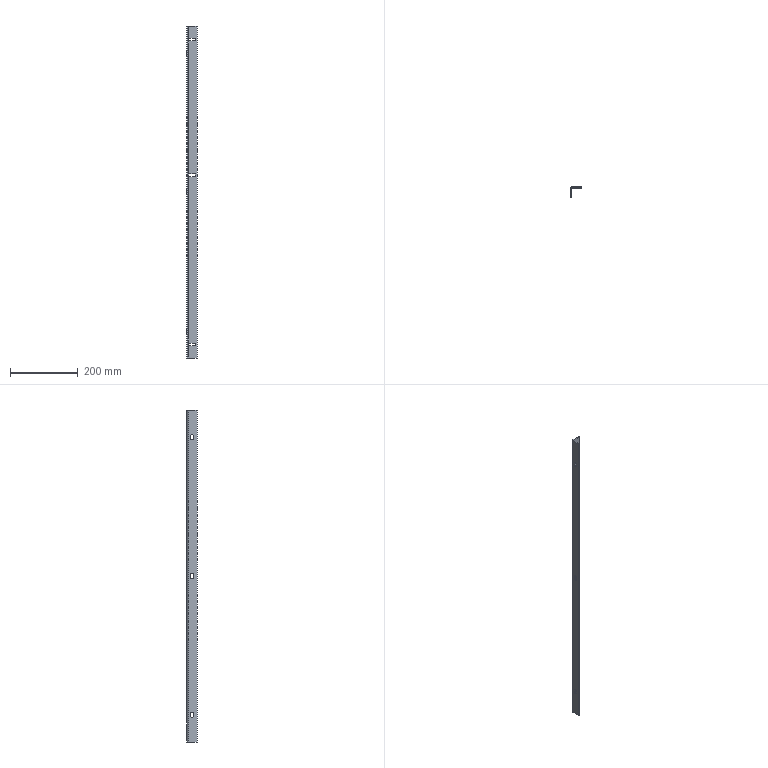Part | NX | features solid 2 | 1 solid | 34 faces | box 30 x 30 x 980 mm | volume 134896 mm3 | plane 26 | cylinder 8 | commonest cylinder face diameters 7 x6 5 x1 10 x1
STEP:
#1=CARTESIAN_POINT('',(-320.,497.5,311.25));
#2=VERTEX_POINT('',#1);
#3=CARTESIAN_POINT('',(-320.,500.,311.25));
#4=VERTEX_POINT('',#3);
#5=CARTESIAN_POINT('',(-320.,-480.918,311.25));
#6=DIRECTION('',(0.,1.,0.));
#7=VECTOR('',#6,1000.);
#8=LINE('',#5,#7);
#9=EDGE_CURVE('',#2,#4,#8,.T.);
#10=ORIENTED_EDGE('',*,*,#9,.T.);
#11=CARTESIAN_POINT('',(-300.,500.,311.25));
#12=VERTEX_POINT('',#11);
#13=CARTESIAN_POINT('',(-320.,500.,311.25));
#14=DIRECTION('',(1.,0.,0.));
#15=VECTOR('',#14,1000.);
#16=LINE('',#13,#15);
#17=EDGE_CURVE('',#4,#12,#16,.T.);
#18=ORIENTED_EDGE('',*,*,#17,.T.);
#19=CARTESIAN_POINT('',(-300.,497.5,311.25));
#20=VERTEX_POINT('',#19);
#21=CARTESIAN_POINT('',(-300.,-480.918,311.25));
#22=DIRECTION('',(0.,1.,0.));
#23=VECTOR('',#22,1000.);
#24=LINE('',#21,#23);
#25=EDGE_CURVE('',#20,#12,#24,.T.);
#26=ORIENTED_EDGE('',*,*,#25,.F.);
#27=CARTESIAN_POINT('',(-295.,497.5,311.25));
#28=DIRECTION('',(1.,0.,0.));
#29=VECTOR('',#28,1000.);
#30=LINE('',#27,#29);
#31=EDGE_CURVE('',#2,#20,#30,.T.);
#32=ORIENTED_EDGE('',*,*,#31,.F.);
#33=EDGE_LOOP('',(#10,#18,#26,#32));
#34=FACE_BOUND('',#33,.T.);
#35=CARTESIAN_POINT('',(-320.,-480.918,311.25));
#36=DIRECTION('',(0.,0.,1.));
#37=DIRECTION('',(1.,0.,0.));
#38=AXIS2_PLACEMENT_3D('',#35,#36,#37);
#39=PLANE('',#38);
#40=ADVANCED_FACE('',(#34),#39,.F.);
#41=CARTESIAN_POINT('',(-320.,497.5,302.75));
#42=VERTEX_POINT('',#41);
#43=CARTESIAN_POINT('',(-320.,500.,302.75));
#44=VERTEX_POINT('',#43);
#45=CARTESIAN_POINT('',(-320.,-480.918,302.75));
#46=DIRECTION('',(0.,1.,0.));
#47=VECTOR('',#46,1000.);
#48=LINE('',#45,#47);
#49=EDGE_CURVE('',#42,#44,#48,.T.);
#50=ORIENTED_EDGE('',*,*,#49,.T.);
#51=CARTESIAN_POINT('',(-320.,500.,311.25));
#52=DIRECTION('',(0.,0.,1.));
#53=VECTOR('',#52,1000.);
#54=LINE('',#51,#53);
#55=EDGE_CURVE('',#44,#4,#54,.T.);
#56=ORIENTED_EDGE('',*,*,#55,.T.);
#57=ORIENTED_EDGE('',*,*,#9,.F.);
#58=CARTESIAN_POINT('',(-320.,497.5,267.));
#59=DIRECTION('',(0.,0.,1.));
#60=VECTOR('',#59,1000.);
#61=LINE('',#58,#60);
#62=EDGE_CURVE('',#42,#2,#61,.T.);
#63=ORIENTED_EDGE('',*,*,#62,.F.);
#64=EDGE_LOOP('',(#50,#56,#57,#63));
#65=FACE_BOUND('',#64,.T.);
#66=CARTESIAN_POINT('',(-320.,-480.918,311.25));
#67=DIRECTION('',(-1.,0.,0.));
#68=DIRECTION('',(0.,1.,0.));
#69=AXIS2_PLACEMENT_3D('',#66,#67,#68);
#70=PLANE('',#69);
#71=ADVANCED_FACE('',(#65),#70,.F.);
#72=CARTESIAN_POINT('',(-300.,497.5,302.75));
#73=VERTEX_POINT('',#72);
#74=CARTESIAN_POINT('',(-300.,500.,302.75));
#75=VERTEX_POINT('',#74);
#76=CARTESIAN_POINT('',(-300.,-480.918,302.75));
#77=DIRECTION('',(0.,1.,0.));
#78=VECTOR('',#77,1000.);
#79=LINE('',#76,#78);
#80=EDGE_CURVE('',#73,#75,#79,.T.);
#81=ORIENTED_EDGE('',*,*,#80,.T.);
#82=CARTESIAN_POINT('',(-320.,500.,302.75));
#83=DIRECTION('',(-1.,0.,0.));
#84=VECTOR('',#83,1000.);
#85=LINE('',#82,#84);
#86=EDGE_CURVE('',#75,#44,#85,.T.);
#87=ORIENTED_EDGE('',*,*,#86,.T.);
#88=ORIENTED_EDGE('',*,*,#49,.F.);
#89=CARTESIAN_POINT('',(-295.,497.5,302.75));
#90=DIRECTION('',(-1.,0.,0.));
#91=VECTOR('',#90,1000.);
#92=LINE('',#89,#91);
#93=EDGE_CURVE('',#73,#42,#92,.T.);
#94=ORIENTED_EDGE('',*,*,#93,.F.);
#95=EDGE_LOOP('',(#81,#87,#88,#94));
#96=FACE_BOUND('',#95,.T.);
#97=CARTESIAN_POINT('',(-320.,-480.918,302.75));
#98=DIRECTION('',(0.,0.,-1.));
#99=DIRECTION('',(0.,-1.,0.));
#100=AXIS2_PLACEMENT_3D('',#97,#98,#99);
#101=PLANE('',#100);
#102=ADVANCED_FACE('',(#96),#101,.F.);
#103=ORIENTED_EDGE('',*,*,#25,.T.);
#104=CARTESIAN_POINT('',(-300.,500.,302.75));
#105=DIRECTION('',(0.,0.,-1.));
#106=VECTOR('',#105,1000.);
#107=LINE('',#104,#106);
#108=EDGE_CURVE('',#12,#75,#107,.T.);
#109=ORIENTED_EDGE('',*,*,#108,.T.);
#110=ORIENTED_EDGE('',*,*,#80,.F.);
#111=CARTESIAN_POINT('',(-300.,497.5,1247.));
#112=DIRECTION('',(0.,0.,-1.));
#113=VECTOR('',#112,1000.);
#114=LINE('',#111,#113);
#115=EDGE_CURVE('',#20,#73,#114,.T.);
#116=ORIENTED_EDGE('',*,*,#115,.F.);
#117=EDGE_LOOP('',(#103,#109,#110,#116));
#118=FACE_BOUND('',#117,.T.);
#119=CARTESIAN_POINT('',(-300.,-480.918,302.75));
#120=DIRECTION('',(1.,0.,0.));
#121=DIRECTION('',(0.,1.,0.));
#122=AXIS2_PLACEMENT_3D('',#119,#120,#121);
#123=PLANE('',#122);
#124=ADVANCED_FACE('',(#118),#123,.F.);
#125=CARTESIAN_POINT('',(-320.,497.5,811.25));
#126=VERTEX_POINT('',#125);
#127=CARTESIAN_POINT('',(-320.,500.,811.25));
#128=VERTEX_POINT('',#127);
#129=CARTESIAN_POINT('',(-320.,-480.918,811.25));
#130=DIRECTION('',(0.,1.,0.));
#131=VECTOR('',#130,1000.);
#132=LINE('',#129,#131);
#133=EDGE_CURVE('',#126,#128,#132,.T.);
#134=ORIENTED_EDGE('',*,*,#133,.T.);
#135=CARTESIAN_POINT('',(-300.,500.,811.25));
#136=VERTEX_POINT('',#135);
#137=CARTESIAN_POINT('',(-320.,500.,811.25));
#138=DIRECTION('',(1.,0.,0.));
#139=VECTOR('',#138,1000.);
#140=LINE('',#137,#139);
#141=EDGE_CURVE('',#128,#136,#140,.T.);
#142=ORIENTED_EDGE('',*,*,#141,.T.);
#143=CARTESIAN_POINT('',(-300.,497.5,811.25));
#144=VERTEX_POINT('',#143);
#145=CARTESIAN_POINT('',(-300.,-480.918,811.25));
#146=DIRECTION('',(0.,1.,0.));
#147=VECTOR('',#146,1000.);
#148=LINE('',#145,#147);
#149=EDGE_CURVE('',#144,#136,#148,.T.);
#150=ORIENTED_EDGE('',*,*,#149,.F.);
#151=CARTESIAN_POINT('',(-295.,497.5,811.25));
#152=DIRECTION('',(1.,0.,0.));
#153=VECTOR('',#152,1000.);
#154=LINE('',#151,#153);
#155=EDGE_CURVE('',#126,#144,#154,.T.);
#156=ORIENTED_EDGE('',*,*,#155,.F.);
#157=EDGE_LOOP('',(#134,#142,#150,#156));
#158=FACE_BOUND('',#157,.T.);
#159=CARTESIAN_POINT('',(-320.,-480.918,811.25));
#160=DIRECTION('',(0.,0.,1.));
#161=DIRECTION('',(1.,0.,0.));
#162=AXIS2_PLACEMENT_3D('',#159,#160,#161);
#163=PLANE('',#162);
#164=ADVANCED_FACE('',(#158),#163,.F.);
#165=CARTESIAN_POINT('',(-320.,497.5,802.75));
#166=VERTEX_POINT('',#165);
#167=CARTESIAN_POINT('',(-320.,500.,802.75));
#168=VERTEX_POINT('',#167);
#169=CARTESIAN_POINT('',(-320.,-480.918,802.75));
#170=DIRECTION('',(0.,1.,0.));
#171=VECTOR('',#170,1000.);
#172=LINE('',#169,#171);
#173=EDGE_CURVE('',#166,#168,#172,.T.);
#174=ORIENTED_EDGE('',*,*,#173,.T.);
#175=CARTESIAN_POINT('',(-320.,500.,811.25));
#176=DIRECTION('',(0.,0.,1.));
#177=VECTOR('',#176,1000.);
#178=LINE('',#175,#177);
#179=EDGE_CURVE('',#168,#128,#178,.T.);
#180=ORIENTED_EDGE('',*,*,#179,.T.);
#181=ORIENTED_EDGE('',*,*,#133,.F.);
#182=CARTESIAN_POINT('',(-320.,497.5,267.));
#183=DIRECTION('',(0.,0.,1.));
#184=VECTOR('',#183,1000.);
#185=LINE('',#182,#184);
#186=EDGE_CURVE('',#166,#126,#185,.T.);
#187=ORIENTED_EDGE('',*,*,#186,.F.);
#188=EDGE_LOOP('',(#174,#180,#181,#187));
#189=FACE_BOUND('',#188,.T.);
#190=CARTESIAN_POINT('',(-320.,-480.918,811.25));
#191=DIRECTION('',(-1.,0.,0.));
#192=DIRECTION('',(0.,1.,0.));
#193=AXIS2_PLACEMENT_3D('',#190,#191,#192);
#194=PLANE('',#193);
#195=ADVANCED_FACE('',(#189),#194,.F.);
#196=CARTESIAN_POINT('',(-300.,497.5,802.75));
#197=VERTEX_POINT('',#196);
#198=CARTESIAN_POINT('',(-300.,500.,802.75));
#199=VERTEX_POINT('',#198);
#200=CARTESIAN_POINT('',(-300.,-480.918,802.75));
#201=DIRECTION('',(0.,1.,0.));
#202=VECTOR('',#201,1000.);
#203=LINE('',#200,#202);
#204=EDGE_CURVE('',#197,#199,#203,.T.);
#205=ORIENTED_EDGE('',*,*,#204,.T.);
#206=CARTESIAN_POINT('',(-320.,500.,802.75));
#207=DIRECTION('',(-1.,0.,0.));
#208=VECTOR('',#207,1000.);
#209=LINE('',#206,#208);
#210=EDGE_CURVE('',#199,#168,#209,.T.);
#211=ORIENTED_EDGE('',*,*,#210,.T.);
#212=ORIENTED_EDGE('',*,*,#173,.F.);
#213=CARTESIAN_POINT('',(-295.,497.5,802.75));
#214=DIRECTION('',(-1.,0.,0.));
#215=VECTOR('',#214,1000.);
#216=LINE('',#213,#215);
#217=EDGE_CURVE('',#197,#166,#216,.T.);
#218=ORIENTED_EDGE('',*,*,#217,.F.);
#219=EDGE_LOOP('',(#205,#211,#212,#218));
#220=FACE_BOUND('',#219,.T.);
#221=CARTESIAN_POINT('',(-320.,-480.918,802.75));
#222=DIRECTION('',(0.,0.,-1.));
#223=DIRECTION('',(0.,-1.,0.));
#224=AXIS2_PLACEMENT_3D('',#221,#222,#223);
#225=PLANE('',#224);
#226=ADVANCED_FACE('',(#220),#225,.F.);
#227=ORIENTED_EDGE('',*,*,#149,.T.);
#228=CARTESIAN_POINT('',(-300.,500.,802.75));
#229=DIRECTION('',(0.,0.,-1.));
#230=VECTOR('',#229,1000.);
#231=LINE('',#228,#230);
#232=EDGE_CURVE('',#136,#199,#231,.T.);
#233=ORIENTED_EDGE('',*,*,#232,.T.);
#234=ORIENTED_EDGE('',*,*,#204,.F.);
#235=CARTESIAN_POINT('',(-300.,497.5,1247.));
#236=DIRECTION('',(0.,0.,-1.));
#237=VECTOR('',#236,1000.);
#238=LINE('',#235,#237);
#239=EDGE_CURVE('',#144,#197,#238,.T.);
#240=ORIENTED_EDGE('',*,*,#239,.F.);
#241=EDGE_LOOP('',(#227,#233,#234,#240));
#242=FACE_BOUND('',#241,.T.);
#243=CARTESIAN_POINT('',(-300.,-480.918,802.75));
#244=DIRECTION('',(1.,0.,0.));
#245=DIRECTION('',(0.,1.,0.));
#246=AXIS2_PLACEMENT_3D('',#243,#244,#245);
#247=PLANE('',#246);
#248=ADVANCED_FACE('',(#242),#247,.F.);
#249=CARTESIAN_POINT('',(-320.,497.5,1211.25));
#250=VERTEX_POINT('',#249);
#251=CARTESIAN_POINT('',(-320.,500.,1211.25));
#252=VERTEX_POINT('',#251);
#253=CARTESIAN_POINT('',(-320.,-480.918,1211.25));
#254=DIRECTION('',(0.,1.,0.));
#255=VECTOR('',#254,1000.);
#256=LINE('',#253,#255);
#257=EDGE_CURVE('',#250,#252,#256,.T.);
#258=ORIENTED_EDGE('',*,*,#257,.T.);
#259=CARTESIAN_POINT('',(-300.,500.,1211.25));
#260=VERTEX_POINT('',#259);
#261=CARTESIAN_POINT('',(-320.,500.,1211.25));
#262=DIRECTION('',(1.,0.,0.));
#263=VECTOR('',#262,1000.);
#264=LINE('',#261,#263);
#265=EDGE_CURVE('',#252,#260,#264,.T.);
#266=ORIENTED_EDGE('',*,*,#265,.T.);
#267=CARTESIAN_POINT('',(-300.,497.5,1211.25));
#268=VERTEX_POINT('',#267);
#269=CARTESIAN_POINT('',(-300.,-480.918,1211.25));
#270=DIRECTION('',(0.,1.,0.));
#271=VECTOR('',#270,1000.);
#272=LINE('',#269,#271);
#273=EDGE_CURVE('',#268,#260,#272,.T.);
#274=ORIENTED_EDGE('',*,*,#273,.F.);
#275=CARTESIAN_POINT('',(-295.,497.5,1211.25));
#276=DIRECTION('',(1.,0.,0.));
#277=VECTOR('',#276,1000.);
#278=LINE('',#275,#277);
#279=EDGE_CURVE('',#250,#268,#278,.T.);
#280=ORIENTED_EDGE('',*,*,#279,.F.);
#281=EDGE_LOOP('',(#258,#266,#274,#280));
#282=FACE_BOUND('',#281,.T.);
#283=CARTESIAN_POINT('',(-320.,-480.918,1211.25));
#284=DIRECTION('',(0.,0.,1.));
#285=DIRECTION('',(1.,0.,0.));
#286=AXIS2_PLACEMENT_3D('',#283,#284,#285);
#287=PLANE('',#286);
#288=ADVANCED_FACE('',(#282),#287,.F.);
#289=CARTESIAN_POINT('',(-320.,497.5,1202.75));
#290=VERTEX_POINT('',#289);
#291=CARTESIAN_POINT('',(-320.,500.,1202.75));
#292=VERTEX_POINT('',#291);
#293=CARTESIAN_POINT('',(-320.,-480.918,1202.75));
#294=DIRECTION('',(0.,1.,0.));
#295=VECTOR('',#294,1000.);
#296=LINE('',#293,#295);
#297=EDGE_CURVE('',#290,#292,#296,.T.);
#298=ORIENTED_EDGE('',*,*,#297,.T.);
#299=CARTESIAN_POINT('',(-320.,500.,1211.25));
#300=DIRECTION('',(0.,0.,1.));
#301=VECTOR('',#300,1000.);
#302=LINE('',#299,#301);
#303=EDGE_CURVE('',#292,#252,#302,.T.);
#304=ORIENTED_EDGE('',*,*,#303,.T.);
#305=ORIENTED_EDGE('',*,*,#257,.F.);
#306=CARTESIAN_POINT('',(-320.,497.5,267.));
#307=DIRECTION('',(0.,0.,1.));
#308=VECTOR('',#307,1000.);
#309=LINE('',#306,#308);
#310=EDGE_CURVE('',#290,#250,#309,.T.);
#311=ORIENTED_EDGE('',*,*,#310,.F.);
#312=EDGE_LOOP('',(#298,#304,#305,#311));
#313=FACE_BOUND('',#312,.T.);
#314=CARTESIAN_POINT('',(-320.,-480.918,1211.25));
#315=DIRECTION('',(-1.,0.,0.));
#316=DIRECTION('',(0.,1.,0.));
#317=AXIS2_PLACEMENT_3D('',#314,#315,#316);
#318=PLANE('',#317);
#319=ADVANCED_FACE('',(#313),#318,.F.);
#320=CARTESIAN_POINT('',(-300.,497.5,1202.75));
#321=VERTEX_POINT('',#320);
#322=CARTESIAN_POINT('',(-300.,500.,1202.75));
#323=VERTEX_POINT('',#322);
#324=CARTESIAN_POINT('',(-300.,-480.918,1202.75));
#325=DIRECTION('',(0.,1.,0.));
#326=VECTOR('',#325,1000.);
#327=LINE('',#324,#326);
#328=EDGE_CURVE('',#321,#323,#327,.T.);
#329=ORIENTED_EDGE('',*,*,#328,.T.);
#330=CARTESIAN_POINT('',(-320.,500.,1202.75));
#331=DIRECTION('',(-1.,0.,0.));
#332=VECTOR('',#331,1000.);
#333=LINE('',#330,#332);
#334=EDGE_CURVE('',#323,#292,#333,.T.);
#335=ORIENTED_EDGE('',*,*,#334,.T.);
#336=ORIENTED_EDGE('',*,*,#297,.F.);
#337=CARTESIAN_POINT('',(-295.,497.5,1202.75));
#338=DIRECTION('',(-1.,0.,0.));
#339=VECTOR('',#338,1000.);
#340=LINE('',#337,#339);
#341=EDGE_CURVE('',#321,#290,#340,.T.);
#342=ORIENTED_EDGE('',*,*,#341,.F.);
#343=EDGE_LOOP('',(#329,#335,#336,#342));
#344=FACE_BOUND('',#343,.T.);
#345=CARTESIAN_POINT('',(-320.,-480.918,1202.75));
#346=DIRECTION('',(0.,0.,-1.));
#347=DIRECTION('',(0.,-1.,0.));
#348=AXIS2_PLACEMENT_3D('',#345,#346,#347);
#349=PLANE('',#348);
#350=ADVANCED_FACE('',(#344),#349,.F.);
#351=ORIENTED_EDGE('',*,*,#273,.T.);
#352=CARTESIAN_POINT('',(-300.,500.,1202.75));
#353=DIRECTION('',(0.,0.,-1.));
#354=VECTOR('',#353,1000.);
#355=LINE('',#352,#354);
#356=EDGE_CURVE('',#260,#323,#355,.T.);
#357=ORIENTED_EDGE('',*,*,#356,.T.);
#358=ORIENTED_EDGE('',*,*,#328,.F.);
#359=CARTESIAN_POINT('',(-300.,497.5,1247.));
#360=DIRECTION('',(0.,0.,-1.));
#361=VECTOR('',#360,1000.);
#362=LINE('',#359,#361);
#363=EDGE_CURVE('',#268,#321,#362,.T.);
#364=ORIENTED_EDGE('',*,*,#363,.F.);
#365=EDGE_LOOP('',(#351,#357,#358,#364));
#366=FACE_BOUND('',#365,.T.);
#367=CARTESIAN_POINT('',(-300.,-480.918,1202.75));
#368=DIRECTION('',(1.,0.,0.));
#369=DIRECTION('',(0.,1.,0.));
#370=AXIS2_PLACEMENT_3D('',#367,#368,#369);
#371=PLANE('',#370);
#372=ADVANCED_FACE('',(#366),#371,.F.);
#373=CARTESIAN_POINT('',(-325.,488.5,351.5));
#374=VERTEX_POINT('',#373);
#375=CARTESIAN_POINT('',(-325.,488.5,342.5));
#376=VERTEX_POINT('',#375);
#377=CARTESIAN_POINT('',(-325.,488.5,267.));
#378=DIRECTION('',(0.,0.,-1.));
#379=VECTOR('',#378,1000.);
#380=LINE('',#377,#379);
#381=EDGE_CURVE('',#374,#376,#380,.T.);
#382=ORIENTED_EDGE('',*,*,#381,.T.);
#383=CARTESIAN_POINT('',(-322.5,488.5,342.5));
#384=VERTEX_POINT('',#383);
#385=CARTESIAN_POINT('',(-1303.418,488.5,342.5));
#386=DIRECTION('',(1.,0.,0.));
#387=VECTOR('',#386,1000.);
#388=LINE('',#385,#387);
#389=EDGE_CURVE('',#376,#384,#388,.T.);
#390=ORIENTED_EDGE('',*,*,#389,.T.);
#391=CARTESIAN_POINT('',(-322.5,488.5,351.5));
#392=VERTEX_POINT('',#391);
#393=CARTESIAN_POINT('',(-322.5,488.5,342.5));
#394=DIRECTION('',(0.,0.,1.));
#395=VECTOR('',#394,1000.);
#396=LINE('',#393,#395);
#397=EDGE_CURVE('',#384,#392,#396,.T.);
#398=ORIENTED_EDGE('',*,*,#397,.T.);
#399=CARTESIAN_POINT('',(-1303.418,488.5,351.5));
#400=DIRECTION('',(1.,0.,0.));
#401=VECTOR('',#400,1000.);
#402=LINE('',#399,#401);
#403=EDGE_CURVE('',#374,#392,#402,.T.);
#404=ORIENTED_EDGE('',*,*,#403,.F.);
#405=EDGE_LOOP('',(#382,#390,#398,#404));
#406=FACE_BOUND('',#405,.T.);
#407=CARTESIAN_POINT('',(-1303.418,488.5,342.5));
#408=DIRECTION('',(0.,1.,0.));
#409=DIRECTION('',(1.,0.,0.));
#410=AXIS2_PLACEMENT_3D('',#407,#408,#409);
#411=PLANE('',#410);
#412=ADVANCED_FACE('',(#406),#411,.F.);
#413=CARTESIAN_POINT('',(-325.,481.5,342.5));
#414=VERTEX_POINT('',#413);
#415=CARTESIAN_POINT('',(-325.,485.,342.5));
#416=DIRECTION('',(-1.,0.,0.));
#417=DIRECTION('',(0.,-1.,0.));
#418=AXIS2_PLACEMENT_3D('',#415,#416,#417);
#419=CIRCLE('',#418,3.5);
#420=EDGE_CURVE('',#376,#414,#419,.T.);
#421=ORIENTED_EDGE('',*,*,#420,.T.);
#422=CARTESIAN_POINT('',(-322.5,481.5,342.5));
#423=VERTEX_POINT('',#422);
#424=CARTESIAN_POINT('',(-1303.418,481.5,342.5));
#425=DIRECTION('',(1.,0.,0.));
#426=VECTOR('',#425,1000.);
#427=LINE('',#424,#426);
#428=EDGE_CURVE('',#414,#423,#427,.T.);
#429=ORIENTED_EDGE('',*,*,#428,.T.);
#430=CARTESIAN_POINT('',(-322.5,485.,342.5));
#431=DIRECTION('',(1.,0.,0.));
#432=DIRECTION('',(0.,-1.,0.));
#433=AXIS2_PLACEMENT_3D('',#430,#431,#432);
#434=CIRCLE('',#433,3.5);
#435=EDGE_CURVE('',#423,#384,#434,.T.);
#436=ORIENTED_EDGE('',*,*,#435,.T.);
#437=ORIENTED_EDGE('',*,*,#389,.F.);
#438=EDGE_LOOP('',(#421,#429,#436,#437));
#439=FACE_BOUND('',#438,.T.);
#440=CARTESIAN_POINT('',(-1303.418,485.,342.5));
#441=DIRECTION('',(1.,0.,0.));
#442=DIRECTION('',(0.,1.,0.));
#443=AXIS2_PLACEMENT_3D('',#440,#441,#442);
#444=CYLINDRICAL_SURFACE('',#443,3.5);
#445=ADVANCED_FACE('',(#439),#444,.F.);
#446=CARTESIAN_POINT('',(-325.,481.5,351.5));
#447=VERTEX_POINT('',#446);
#448=CARTESIAN_POINT('',(-325.,481.5,267.));
#449=DIRECTION('',(0.,0.,1.));
#450=VECTOR('',#449,1000.);
#451=LINE('',#448,#450);
#452=EDGE_CURVE('',#414,#447,#451,.T.);
#453=ORIENTED_EDGE('',*,*,#452,.T.);
#454=CARTESIAN_POINT('',(-322.5,481.5,351.5));
#455=VERTEX_POINT('',#454);
#456=CARTESIAN_POINT('',(-1303.418,481.5,351.5));
#457=DIRECTION('',(1.,0.,0.));
#458=VECTOR('',#457,1000.);
#459=LINE('',#456,#458);
#460=EDGE_CURVE('',#447,#455,#459,.T.);
#461=ORIENTED_EDGE('',*,*,#460,.T.);
#462=CARTESIAN_POINT('',(-322.5,481.5,342.5));
#463=DIRECTION('',(0.,0.,-1.));
#464=VECTOR('',#463,1000.);
#465=LINE('',#462,#464);
#466=EDGE_CURVE('',#455,#423,#465,.T.);
#467=ORIENTED_EDGE('',*,*,#466,.T.);
#468=ORIENTED_EDGE('',*,*,#428,.F.);
#469=EDGE_LOOP('',(#453,#461,#467,#468));
#470=FACE_BOUND('',#469,.T.);
#471=CARTESIAN_POINT('',(-1303.418,481.5,342.5));
#472=DIRECTION('',(0.,-1.,0.));
#473=DIRECTION('',(0.,0.,-1.));
#474=AXIS2_PLACEMENT_3D('',#471,#472,#473);
#475=PLANE('',#474);
#476=ADVANCED_FACE('',(#470),#475,.F.);
#477=CARTESIAN_POINT('',(-325.,485.,351.5));
#478=DIRECTION('',(-1.,0.,0.));
#479=DIRECTION('',(0.,-1.,0.));
#480=AXIS2_PLACEMENT_3D('',#477,#478,#479);
#481=CIRCLE('',#480,3.5);
#482=EDGE_CURVE('',#447,#374,#481,.T.);
#483=ORIENTED_EDGE('',*,*,#482,.T.);
#484=ORIENTED_EDGE('',*,*,#403,.T.);
#485=CARTESIAN_POINT('',(-322.5,485.,351.5));
#486=DIRECTION('',(1.,0.,0.));
#487=DIRECTION('',(0.,1.,0.));
#488=AXIS2_PLACEMENT_3D('',#485,#486,#487);
#489=CIRCLE('',#488,3.5);
#490=EDGE_CURVE('',#392,#455,#489,.T.);
#491=ORIENTED_EDGE('',*,*,#490,.T.);
#492=ORIENTED_EDGE('',*,*,#460,.F.);
#493=EDGE_LOOP('',(#483,#484,#491,#492));
#494=FACE_BOUND('',#493,.T.);
#495=CARTESIAN_POINT('',(-1303.418,485.,351.5));
#496=DIRECTION('',(1.,0.,0.));
#497=DIRECTION('',(0.,1.,0.));
#498=AXIS2_PLACEMENT_3D('',#495,#496,#497);
#499=CYLINDRICAL_SURFACE('',#498,3.5);
#500=ADVANCED_FACE('',(#494),#499,.F.);
#501=CARTESIAN_POINT('',(-325.,481.5,752.5));
#502=VERTEX_POINT('',#501);
#503=CARTESIAN_POINT('',(-325.,481.5,761.5));
#504=VERTEX_POINT('',#503);
#505=CARTESIAN_POINT('',(-325.,481.5,267.));
#506=DIRECTION('',(0.,0.,1.));
#507=VECTOR('',#506,1000.);
#508=LINE('',#505,#507);
#509=EDGE_CURVE('',#502,#504,#508,.T.);
#510=ORIENTED_EDGE('',*,*,#509,.T.);
#511=CARTESIAN_POINT('',(-322.5,481.5,761.5));
#512=VERTEX_POINT('',#511);
#513=CARTESIAN_POINT('',(-1303.418,481.5,761.5));
#514=DIRECTION('',(1.,0.,0.));
#515=VECTOR('',#514,1000.);
#516=LINE('',#513,#515);
#517=EDGE_CURVE('',#504,#512,#516,.T.);
#518=ORIENTED_EDGE('',*,*,#517,.T.);
#519=CARTESIAN_POINT('',(-322.5,481.5,752.5));
#520=VERTEX_POINT('',#519);
#521=CARTESIAN_POINT('',(-322.5,481.5,761.5));
#522=DIRECTION('',(0.,0.,-1.));
#523=VECTOR('',#522,1000.);
#524=LINE('',#521,#523);
#525=EDGE_CURVE('',#512,#520,#524,.T.);
#526=ORIENTED_EDGE('',*,*,#525,.T.);
#527=CARTESIAN_POINT('',(-1303.418,481.5,752.5));
#528=DIRECTION('',(1.,0.,0.));
#529=VECTOR('',#528,1000.);
#530=LINE('',#527,#529);
#531=EDGE_CURVE('',#502,#520,#530,.T.);
#532=ORIENTED_EDGE('',*,*,#531,.F.);
#533=EDGE_LOOP('',(#510,#518,#526,#532));
#534=FACE_BOUND('',#533,.T.);
#535=CARTESIAN_POINT('',(-1303.418,481.5,761.5));
#536=DIRECTION('',(0.,-1.,0.));
#537=DIRECTION('',(0.,0.,-1.));
#538=AXIS2_PLACEMENT_3D('',#535,#536,#537);
#539=PLANE('',#538);
#540=ADVANCED_FACE('',(#534),#539,.F.);
#541=CARTESIAN_POINT('',(-325.,488.5,761.5));
#542=VERTEX_POINT('',#541);
#543=CARTESIAN_POINT('',(-325.,485.,761.5));
#544=DIRECTION('',(-1.,0.,0.));
#545=DIRECTION('',(0.,-1.,0.));
#546=AXIS2_PLACEMENT_3D('',#543,#544,#545);
#547=CIRCLE('',#546,3.5);
#548=EDGE_CURVE('',#504,#542,#547,.T.);
#549=ORIENTED_EDGE('',*,*,#548,.T.);
#550=CARTESIAN_POINT('',(-322.5,488.5,761.5));
#551=VERTEX_POINT('',#550);
#552=CARTESIAN_POINT('',(-1303.418,488.5,761.5));
#553=DIRECTION('',(1.,0.,0.));
#554=VECTOR('',#553,1000.);
#555=LINE('',#552,#554);
#556=EDGE_CURVE('',#542,#551,#555,.T.);
#557=ORIENTED_EDGE('',*,*,#556,.T.);
#558=CARTESIAN_POINT('',(-322.5,485.,761.5));
#559=DIRECTION('',(1.,0.,0.));
#560=DIRECTION('',(0.,1.,0.));
#561=AXIS2_PLACEMENT_3D('',#558,#559,#560);
#562=CIRCLE('',#561,3.5);
#563=EDGE_CURVE('',#551,#512,#562,.T.);
#564=ORIENTED_EDGE('',*,*,#563,.T.);
#565=ORIENTED_EDGE('',*,*,#517,.F.);
#566=EDGE_LOOP('',(#549,#557,#564,#565));
#567=FACE_BOUND('',#566,.T.);
#568=CARTESIAN_POINT('',(-1303.418,485.,761.5));
#569=DIRECTION('',(1.,0.,0.));
#570=DIRECTION('',(0.,1.,0.));
#571=AXIS2_PLACEMENT_3D('',#568,#569,#570);
#572=CYLINDRICAL_SURFACE('',#571,3.5);
#573=ADVANCED_FACE('',(#567),#572,.F.);
#574=CARTESIAN_POINT('',(-325.,488.5,752.5));
#575=VERTEX_POINT('',#574);
#576=CARTESIAN_POINT('',(-325.,488.5,267.));
#577=DIRECTION('',(0.,0.,-1.));
#578=VECTOR('',#577,1000.);
#579=LINE('',#576,#578);
#580=EDGE_CURVE('',#542,#575,#579,.T.);
#581=ORIENTED_EDGE('',*,*,#580,.T.);
#582=CARTESIAN_POINT('',(-322.5,488.5,752.5));
#583=VERTEX_POINT('',#582);
#584=CARTESIAN_POINT('',(-1303.418,488.5,752.5));
#585=DIRECTION('',(1.,0.,0.));
#586=VECTOR('',#585,1000.);
#587=LINE('',#584,#586);
#588=EDGE_CURVE('',#575,#583,#587,.T.);
#589=ORIENTED_EDGE('',*,*,#588,.T.);
#590=CARTESIAN_POINT('',(-322.5,488.5,761.5));
#591=DIRECTION('',(0.,0.,1.));
#592=VECTOR('',#591,1000.);
#593=LINE('',#590,#592);
#594=EDGE_CURVE('',#583,#551,#593,.T.);
#595=ORIENTED_EDGE('',*,*,#594,.T.);
#596=ORIENTED_EDGE('',*,*,#556,.F.);
#597=EDGE_LOOP('',(#581,#589,#595,#596));
#598=FACE_BOUND('',#597,.T.);
#599=CARTESIAN_POINT('',(-1303.418,488.5,761.5));
#600=DIRECTION('',(0.,1.,0.));
#601=DIRECTION('',(1.,0.,0.));
#602=AXIS2_PLACEMENT_3D('',#599,#600,#601);
#603=PLANE('',#602);
#604=ADVANCED_FACE('',(#598),#603,.F.);
#605=CARTESIAN_POINT('',(-325.,485.,752.5));
#606=DIRECTION('',(-1.,0.,0.));
#607=DIRECTION('',(0.,-1.,0.));
#608=AXIS2_PLACEMENT_3D('',#605,#606,#607);
#609=CIRCLE('',#608,3.5);
#610=EDGE_CURVE('',#575,#502,#609,.T.);
#611=ORIENTED_EDGE('',*,*,#610,.T.);
#612=ORIENTED_EDGE('',*,*,#531,.T.);
#613=CARTESIAN_POINT('',(-322.5,485.,752.5));
#614=DIRECTION('',(1.,0.,0.));
#615=DIRECTION('',(0.,-1.,0.));
#616=AXIS2_PLACEMENT_3D('',#613,#614,#615);
#617=CIRCLE('',#616,3.5);
#618=EDGE_CURVE('',#520,#583,#617,.T.);
#619=ORIENTED_EDGE('',*,*,#618,.T.);
#620=ORIENTED_EDGE('',*,*,#588,.F.);
#621=EDGE_LOOP('',(#611,#612,#619,#620));
#622=FACE_BOUND('',#621,.T.);
#623=CARTESIAN_POINT('',(-1303.418,485.,752.5));
#624=DIRECTION('',(1.,0.,0.));
#625=DIRECTION('',(0.,1.,0.));
#626=AXIS2_PLACEMENT_3D('',#623,#624,#625);
#627=CYLINDRICAL_SURFACE('',#626,3.5);
#628=ADVANCED_FACE('',(#622),#627,.F.);
#629=CARTESIAN_POINT('',(-325.,488.5,1171.5));
#630=VERTEX_POINT('',#629);
#631=CARTESIAN_POINT('',(-325.,488.5,1162.5));
#632=VERTEX_POINT('',#631);
#633=CARTESIAN_POINT('',(-325.,488.5,267.));
#634=DIRECTION('',(0.,0.,-1.));
#635=VECTOR('',#634,1000.);
#636=LINE('',#633,#635);
#637=EDGE_CURVE('',#630,#632,#636,.T.);
#638=ORIENTED_EDGE('',*,*,#637,.T.);
#639=CARTESIAN_POINT('',(-322.5,488.5,1162.5));
#640=VERTEX_POINT('',#639);
#641=CARTESIAN_POINT('',(-1303.418,488.5,1162.5));
#642=DIRECTION('',(1.,0.,0.));
#643=VECTOR('',#642,1000.);
#644=LINE('',#641,#643);
#645=EDGE_CURVE('',#632,#640,#644,.T.);
#646=ORIENTED_EDGE('',*,*,#645,.T.);
#647=CARTESIAN_POINT('',(-322.5,488.5,1171.5));
#648=VERTEX_POINT('',#647);
#649=CARTESIAN_POINT('',(-322.5,488.5,1162.5));
#650=DIRECTION('',(0.,0.,1.));
#651=VECTOR('',#650,1000.);
#652=LINE('',#649,#651);
#653=EDGE_CURVE('',#640,#648,#652,.T.);
#654=ORIENTED_EDGE('',*,*,#653,.T.);
#655=CARTESIAN_POINT('',(-1303.418,488.5,1171.5));
#656=DIRECTION('',(1.,0.,0.));
#657=VECTOR('',#656,1000.);
#658=LINE('',#655,#657);
#659=EDGE_CURVE('',#630,#648,#658,.T.);
#660=ORIENTED_EDGE('',*,*,#659,.F.);
#661=EDGE_LOOP('',(#638,#646,#654,#660));
#662=FACE_BOUND('',#661,.T.);
#663=CARTESIAN_POINT('',(-1303.418,488.5,1162.5));
#664=DIRECTION('',(0.,1.,0.));
#665=DIRECTION('',(1.,0.,0.));
#666=AXIS2_PLACEMENT_3D('',#663,#664,#665);
#667=PLANE('',#666);
#668=ADVANCED_FACE('',(#662),#667,.F.);
#669=CARTESIAN_POINT('',(-325.,481.5,1162.5));
#670=VERTEX_POINT('',#669);
#671=CARTESIAN_POINT('',(-325.,485.,1162.5));
#672=DIRECTION('',(-1.,0.,0.));
#673=DIRECTION('',(0.,-1.,0.));
#674=AXIS2_PLACEMENT_3D('',#671,#672,#673);
#675=CIRCLE('',#674,3.5);
#676=EDGE_CURVE('',#632,#670,#675,.T.);
#677=ORIENTED_EDGE('',*,*,#676,.T.);
#678=CARTESIAN_POINT('',(-322.5,481.5,1162.5));
#679=VERTEX_POINT('',#678);
#680=CARTESIAN_POINT('',(-1303.418,481.5,1162.5));
#681=DIRECTION('',(1.,0.,0.));
#682=VECTOR('',#681,1000.);
#683=LINE('',#680,#682);
#684=EDGE_CURVE('',#670,#679,#683,.T.);
#685=ORIENTED_EDGE('',*,*,#684,.T.);
#686=CARTESIAN_POINT('',(-322.5,485.,1162.5));
#687=DIRECTION('',(1.,0.,0.));
#688=DIRECTION('',(0.,-1.,0.));
#689=AXIS2_PLACEMENT_3D('',#686,#687,#688);
#690=CIRCLE('',#689,3.5);
#691=EDGE_CURVE('',#679,#640,#690,.T.);
#692=ORIENTED_EDGE('',*,*,#691,.T.);
#693=ORIENTED_EDGE('',*,*,#645,.F.);
#694=EDGE_LOOP('',(#677,#685,#692,#693));
#695=FACE_BOUND('',#694,.T.);
#696=CARTESIAN_POINT('',(-1303.418,485.,1162.5));
#697=DIRECTION('',(1.,0.,0.));
#698=DIRECTION('',(0.,1.,0.));
#699=AXIS2_PLACEMENT_3D('',#696,#697,#698);
#700=CYLINDRICAL_SURFACE('',#699,3.5);
#701=ADVANCED_FACE('',(#695),#700,.F.);
#702=CARTESIAN_POINT('',(-325.,481.5,1171.5));
#703=VERTEX_POINT('',#702);
#704=CARTESIAN_POINT('',(-325.,481.5,267.));
#705=DIRECTION('',(0.,0.,1.));
#706=VECTOR('',#705,1000.);
#707=LINE('',#704,#706);
#708=EDGE_CURVE('',#670,#703,#707,.T.);
#709=ORIENTED_EDGE('',*,*,#708,.T.);
#710=CARTESIAN_POINT('',(-322.5,481.5,1171.5));
#711=VERTEX_POINT('',#710);
#712=CARTESIAN_POINT('',(-1303.418,481.5,1171.5));
#713=DIRECTION('',(1.,0.,0.));
#714=VECTOR('',#713,1000.);
#715=LINE('',#712,#714);
#716=EDGE_CURVE('',#703,#711,#715,.T.);
#717=ORIENTED_EDGE('',*,*,#716,.T.);
#718=CARTESIAN_POINT('',(-322.5,481.5,1162.5));
#719=DIRECTION('',(0.,0.,-1.));
#720=VECTOR('',#719,1000.);
#721=LINE('',#718,#720);
#722=EDGE_CURVE('',#711,#679,#721,.T.);
#723=ORIENTED_EDGE('',*,*,#722,.T.);
#724=ORIENTED_EDGE('',*,*,#684,.F.);
#725=EDGE_LOOP('',(#709,#717,#723,#724));
#726=FACE_BOUND('',#725,.T.);
#727=CARTESIAN_POINT('',(-1303.418,481.5,1162.5));
#728=DIRECTION('',(0.,-1.,0.));
#729=DIRECTION('',(0.,0.,-1.));
#730=AXIS2_PLACEMENT_3D('',#727,#728,#729);
#731=PLANE('',#730);
#732=ADVANCED_FACE('',(#726),#731,.F.);
#733=CARTESIAN_POINT('',(-325.,485.,1171.5));
#734=DIRECTION('',(-1.,0.,0.));
#735=DIRECTION('',(0.,-1.,0.));
#736=AXIS2_PLACEMENT_3D('',#733,#734,#735);
#737=CIRCLE('',#736,3.5);
#738=EDGE_CURVE('',#703,#630,#737,.T.);
#739=ORIENTED_EDGE('',*,*,#738,.T.);
#740=ORIENTED_EDGE('',*,*,#659,.T.);
#741=CARTESIAN_POINT('',(-322.5,485.,1171.5));
#742=DIRECTION('',(1.,0.,0.));
#743=DIRECTION('',(0.,1.,0.));
#744=AXIS2_PLACEMENT_3D('',#741,#742,#743);
#745=CIRCLE('',#744,3.5);
#746=EDGE_CURVE('',#648,#711,#745,.T.);
#747=ORIENTED_EDGE('',*,*,#746,.T.);
#748=ORIENTED_EDGE('',*,*,#716,.F.);
#749=EDGE_LOOP('',(#739,#740,#747,#748));
#750=FACE_BOUND('',#749,.T.);
#751=CARTESIAN_POINT('',(-1303.418,485.,1171.5));
#752=DIRECTION('',(1.,0.,0.));
#753=DIRECTION('',(0.,1.,0.));
#754=AXIS2_PLACEMENT_3D('',#751,#752,#753);
#755=CYLINDRICAL_SURFACE('',#754,3.5);
#756=ADVANCED_FACE('',(#750),#755,.F.);
#757=CARTESIAN_POINT('',(-322.5,495.,1247.));
#758=VERTEX_POINT('',#757);
#759=CARTESIAN_POINT('',(-320.,497.5,1247.));
#760=VERTEX_POINT('',#759);
#761=CARTESIAN_POINT('',(-320.,495.,1247.));
#762=DIRECTION('',(0.,0.,-1.));
#763=DIRECTION('',(0.,1.,0.));
#764=AXIS2_PLACEMENT_3D('',#761,#762,#763);
#765=CIRCLE('',#764,2.5);
#766=EDGE_CURVE('',#758,#760,#765,.T.);
#767=ORIENTED_EDGE('',*,*,#766,.F.);
#768=CARTESIAN_POINT('',(-322.5,495.,267.));
#769=VERTEX_POINT('',#768);
#770=CARTESIAN_POINT('',(-322.5,495.,267.));
#771=DIRECTION('',(0.,0.,1.));
#772=VECTOR('',#771,1000.);
#773=LINE('',#770,#772);
#774=EDGE_CURVE('',#769,#758,#773,.T.);
#775=ORIENTED_EDGE('',*,*,#774,.F.);
#776=CARTESIAN_POINT('',(-320.,497.5,267.));
#777=VERTEX_POINT('',#776);
#778=CARTESIAN_POINT('',(-320.,495.,267.));
#779=DIRECTION('',(0.,0.,1.));
#780=DIRECTION('',(0.,1.,0.));
#781=AXIS2_PLACEMENT_3D('',#778,#779,#780);
#782=CIRCLE('',#781,2.5);
#783=EDGE_CURVE('',#777,#769,#782,.T.);
#784=ORIENTED_EDGE('',*,*,#783,.F.);
#785=CARTESIAN_POINT('',(-320.,497.5,267.));
#786=DIRECTION('',(0.,0.,1.));
#787=VECTOR('',#786,1000.);
#788=LINE('',#785,#787);
#789=EDGE_CURVE('',#777,#42,#788,.T.);
#790=ORIENTED_EDGE('',*,*,#789,.T.);
#791=ORIENTED_EDGE('',*,*,#62,.T.);
#792=CARTESIAN_POINT('',(-320.,497.5,267.));
#793=DIRECTION('',(0.,0.,1.));
#794=VECTOR('',#793,1000.);
#795=LINE('',#792,#794);
#796=EDGE_CURVE('',#2,#166,#795,.T.);
#797=ORIENTED_EDGE('',*,*,#796,.T.);
#798=ORIENTED_EDGE('',*,*,#186,.T.);
#799=CARTESIAN_POINT('',(-320.,497.5,267.));
#800=DIRECTION('',(0.,0.,1.));
#801=VECTOR('',#800,1000.);
#802=LINE('',#799,#801);
#803=EDGE_CURVE('',#126,#290,#802,.T.);
#804=ORIENTED_EDGE('',*,*,#803,.T.);
#805=ORIENTED_EDGE('',*,*,#310,.T.);
#806=CARTESIAN_POINT('',(-320.,497.5,267.));
#807=DIRECTION('',(0.,0.,1.));
#808=VECTOR('',#807,1000.);
#809=LINE('',#806,#808);
#810=EDGE_CURVE('',#250,#760,#809,.T.);
#811=ORIENTED_EDGE('',*,*,#810,.T.);
#812=EDGE_LOOP('',(#767,#775,#784,#790,#791,#797,#798,#804,#805,#811));
#813=FACE_BOUND('',#812,.T.);
#814=CARTESIAN_POINT('',(-320.,495.,267.));
#815=DIRECTION('',(0.,0.,-1.));
#816=DIRECTION('',(0.,-1.,0.));
#817=AXIS2_PLACEMENT_3D('',#814,#815,#816);
#818=CYLINDRICAL_SURFACE('',#817,2.5);
#819=ADVANCED_FACE('',(#813),#818,.F.);
#820=CARTESIAN_POINT('',(-325.,495.,1247.));
#821=VERTEX_POINT('',#820);
#822=CARTESIAN_POINT('',(-320.,500.,1247.));
#823=VERTEX_POINT('',#822);
#824=CARTESIAN_POINT('',(-320.,495.,1247.));
#825=DIRECTION('',(0.,0.,-1.));
#826=DIRECTION('',(0.,-1.,0.));
#827=AXIS2_PLACEMENT_3D('',#824,#825,#826);
#828=CIRCLE('',#827,5.);
#829=EDGE_CURVE('',#821,#823,#828,.T.);
#830=ORIENTED_EDGE('',*,*,#829,.T.);
#831=CARTESIAN_POINT('',(-320.,500.,1247.));
#832=DIRECTION('',(0.,0.,1.));
#833=VECTOR('',#832,1000.);
#834=LINE('',#831,#833);
#835=EDGE_CURVE('',#252,#823,#834,.T.);
#836=ORIENTED_EDGE('',*,*,#835,.F.);
#837=ORIENTED_EDGE('',*,*,#303,.F.);
#838=CARTESIAN_POINT('',(-320.,500.,1247.));
#839=DIRECTION('',(0.,0.,1.));
#840=VECTOR('',#839,1000.);
#841=LINE('',#838,#840);
#842=EDGE_CURVE('',#128,#292,#841,.T.);
#843=ORIENTED_EDGE('',*,*,#842,.F.);
#844=ORIENTED_EDGE('',*,*,#179,.F.);
#845=CARTESIAN_POINT('',(-320.,500.,1247.));
#846=DIRECTION('',(0.,0.,1.));
#847=VECTOR('',#846,1000.);
#848=LINE('',#845,#847);
#849=EDGE_CURVE('',#4,#168,#848,.T.);
#850=ORIENTED_EDGE('',*,*,#849,.F.);
#851=ORIENTED_EDGE('',*,*,#55,.F.);
#852=CARTESIAN_POINT('',(-320.,500.,267.));
#853=VERTEX_POINT('',#852);
#854=CARTESIAN_POINT('',(-320.,500.,1247.));
#855=DIRECTION('',(0.,0.,1.));
#856=VECTOR('',#855,1000.);
#857=LINE('',#854,#856);
#858=EDGE_CURVE('',#853,#44,#857,.T.);
#859=ORIENTED_EDGE('',*,*,#858,.F.);
#860=CARTESIAN_POINT('',(-325.,495.,267.));
#861=VERTEX_POINT('',#860);
#862=CARTESIAN_POINT('',(-320.,495.,267.));
#863=DIRECTION('',(0.,0.,1.));
#864=DIRECTION('',(0.,-1.,0.));
#865=AXIS2_PLACEMENT_3D('',#862,#863,#864);
#866=CIRCLE('',#865,5.);
#867=EDGE_CURVE('',#853,#861,#866,.T.);
#868=ORIENTED_EDGE('',*,*,#867,.T.);
#869=CARTESIAN_POINT('',(-325.,495.,267.));
#870=DIRECTION('',(0.,0.,1.));
#871=VECTOR('',#870,1000.);
#872=LINE('',#869,#871);
#873=EDGE_CURVE('',#861,#821,#872,.T.);
#874=ORIENTED_EDGE('',*,*,#873,.T.);
#875=EDGE_LOOP('',(#830,#836,#837,#843,#844,#850,#851,#859,#868,#874));
#876=FACE_BOUND('',#875,.T.);
#877=CARTESIAN_POINT('',(-320.,495.,267.));
#878=DIRECTION('',(0.,0.,-1.));
#879=DIRECTION('',(0.,-1.,0.));
#880=AXIS2_PLACEMENT_3D('',#877,#878,#879);
#881=CYLINDRICAL_SURFACE('',#880,5.);
#882=ADVANCED_FACE('',(#876),#881,.T.);
#883=ORIENTED_EDGE('',*,*,#722,.F.);
#884=ORIENTED_EDGE('',*,*,#746,.F.);
#885=ORIENTED_EDGE('',*,*,#653,.F.);
#886=ORIENTED_EDGE('',*,*,#691,.F.);
#887=EDGE_LOOP('',(#883,#884,#885,#886));
#888=FACE_BOUND('',#887,.T.);
#889=ORIENTED_EDGE('',*,*,#594,.F.);
#890=ORIENTED_EDGE('',*,*,#618,.F.);
#891=ORIENTED_EDGE('',*,*,#525,.F.);
#892=ORIENTED_EDGE('',*,*,#563,.F.);
#893=EDGE_LOOP('',(#889,#890,#891,#892));
#894=FACE_BOUND('',#893,.T.);
#895=ORIENTED_EDGE('',*,*,#466,.F.);
#896=ORIENTED_EDGE('',*,*,#490,.F.);
#897=ORIENTED_EDGE('',*,*,#397,.F.);
#898=ORIENTED_EDGE('',*,*,#435,.F.);
#899=EDGE_LOOP('',(#895,#896,#897,#898));
#900=FACE_BOUND('',#899,.T.);
#901=CARTESIAN_POINT('',(-322.5,470.,1247.));
#902=VERTEX_POINT('',#901);
#903=CARTESIAN_POINT('',(-322.5,500.,1247.));
#904=DIRECTION('',(0.,-1.,0.));
#905=VECTOR('',#904,1000.);
#906=LINE('',#903,#905);
#907=EDGE_CURVE('',#758,#902,#906,.T.);
#908=ORIENTED_EDGE('',*,*,#907,.T.);
#909=CARTESIAN_POINT('',(-322.5,470.,267.));
#910=VERTEX_POINT('',#909);
#911=CARTESIAN_POINT('',(-322.5,470.,267.));
#912=DIRECTION('',(0.,0.,1.));
#913=VECTOR('',#912,1000.);
#914=LINE('',#911,#913);
#915=EDGE_CURVE('',#910,#902,#914,.T.);
#916=ORIENTED_EDGE('',*,*,#915,.F.);
#917=CARTESIAN_POINT('',(-322.5,500.,267.));
#918=DIRECTION('',(0.,-1.,0.));
#919=VECTOR('',#918,1000.);
#920=LINE('',#917,#919);
#921=EDGE_CURVE('',#769,#910,#920,.T.);
#922=ORIENTED_EDGE('',*,*,#921,.F.);
#923=ORIENTED_EDGE('',*,*,#774,.T.);
#924=EDGE_LOOP('',(#908,#916,#922,#923));
#925=FACE_BOUND('',#924,.T.);
#926=CARTESIAN_POINT('',(-322.5,500.,267.));
#927=DIRECTION('',(-1.,0.,0.));
#928=DIRECTION('',(0.,1.,0.));
#929=AXIS2_PLACEMENT_3D('',#926,#927,#928);
#930=PLANE('',#929);
#931=ADVANCED_FACE('',(#888,#894,#900,#925),#930,.F.);
#932=ORIENTED_EDGE('',*,*,#738,.F.);
#933=ORIENTED_EDGE('',*,*,#708,.F.);
#934=ORIENTED_EDGE('',*,*,#676,.F.);
#935=ORIENTED_EDGE('',*,*,#637,.F.);
#936=EDGE_LOOP('',(#932,#933,#934,#935));
#937=FACE_BOUND('',#936,.T.);
#938=ORIENTED_EDGE('',*,*,#610,.F.);
#939=ORIENTED_EDGE('',*,*,#580,.F.);
#940=ORIENTED_EDGE('',*,*,#548,.F.);
#941=ORIENTED_EDGE('',*,*,#509,.F.);
#942=EDGE_LOOP('',(#938,#939,#940,#941));
#943=FACE_BOUND('',#942,.T.);
#944=ORIENTED_EDGE('',*,*,#482,.F.);
#945=ORIENTED_EDGE('',*,*,#452,.F.);
#946=ORIENTED_EDGE('',*,*,#420,.F.);
#947=ORIENTED_EDGE('',*,*,#381,.F.);
#948=EDGE_LOOP('',(#944,#945,#946,#947));
#949=FACE_BOUND('',#948,.T.);
#950=CARTESIAN_POINT('',(-325.,470.,1247.));
#951=VERTEX_POINT('',#950);
#952=CARTESIAN_POINT('',(-325.,500.,1247.));
#953=DIRECTION('',(0.,-1.,0.));
#954=VECTOR('',#953,1000.);
#955=LINE('',#952,#954);
#956=EDGE_CURVE('',#821,#951,#955,.T.);
#957=ORIENTED_EDGE('',*,*,#956,.F.);
#958=ORIENTED_EDGE('',*,*,#873,.F.);
#959=CARTESIAN_POINT('',(-325.,470.,267.));
#960=VERTEX_POINT('',#959);
#961=CARTESIAN_POINT('',(-325.,500.,267.));
#962=DIRECTION('',(0.,-1.,0.));
#963=VECTOR('',#962,1000.);
#964=LINE('',#961,#963);
#965=EDGE_CURVE('',#861,#960,#964,.T.);
#966=ORIENTED_EDGE('',*,*,#965,.T.);
#967=CARTESIAN_POINT('',(-325.,470.,267.));
#968=DIRECTION('',(0.,0.,1.));
#969=VECTOR('',#968,1000.);
#970=LINE('',#967,#969);
#971=EDGE_CURVE('',#960,#951,#970,.T.);
#972=ORIENTED_EDGE('',*,*,#971,.T.);
#973=EDGE_LOOP('',(#957,#958,#966,#972));
#974=FACE_BOUND('',#973,.T.);
#975=CARTESIAN_POINT('',(-325.,500.,267.));
#976=DIRECTION('',(-1.,0.,0.));
#977=DIRECTION('',(0.,1.,0.));
#978=AXIS2_PLACEMENT_3D('',#975,#976,#977);
#979=PLANE('',#978);
#980=ADVANCED_FACE('',(#937,#943,#949,#974),#979,.T.);
#981=CARTESIAN_POINT('',(-325.,470.,267.));
#982=DIRECTION('',(-1.,0.,0.));
#983=VECTOR('',#982,1000.);
#984=LINE('',#981,#983);
#985=EDGE_CURVE('',#910,#960,#984,.T.);
#986=ORIENTED_EDGE('',*,*,#985,.F.);
#987=ORIENTED_EDGE('',*,*,#915,.T.);
#988=CARTESIAN_POINT('',(-325.,470.,1247.));
#989=DIRECTION('',(-1.,0.,0.));
#990=VECTOR('',#989,1000.);
#991=LINE('',#988,#990);
#992=EDGE_CURVE('',#902,#951,#991,.T.);
#993=ORIENTED_EDGE('',*,*,#992,.T.);
#994=ORIENTED_EDGE('',*,*,#971,.F.);
#995=EDGE_LOOP('',(#986,#987,#993,#994));
#996=FACE_BOUND('',#995,.T.);
#997=CARTESIAN_POINT('',(-325.,470.,267.));
#998=DIRECTION('',(0.,-1.,0.));
#999=DIRECTION('',(0.,0.,-1.));
#1000=AXIS2_PLACEMENT_3D('',#997,#998,#999);
#1001=PLANE('',#1000);
#1002=ADVANCED_FACE('',(#996),#1001,.T.);
#1003=ORIENTED_EDGE('',*,*,#86,.F.);
#1004=ORIENTED_EDGE('',*,*,#108,.F.);
#1005=ORIENTED_EDGE('',*,*,#17,.F.);
#1006=ORIENTED_EDGE('',*,*,#849,.T.);
#1007=ORIENTED_EDGE('',*,*,#210,.F.);
#1008=ORIENTED_EDGE('',*,*,#232,.F.);
#1009=ORIENTED_EDGE('',*,*,#141,.F.);
#1010=ORIENTED_EDGE('',*,*,#842,.T.);
#1011=ORIENTED_EDGE('',*,*,#334,.F.);
#1012=ORIENTED_EDGE('',*,*,#356,.F.);
#1013=ORIENTED_EDGE('',*,*,#265,.F.);
#1014=ORIENTED_EDGE('',*,*,#835,.T.);
#1015=CARTESIAN_POINT('',(-295.,500.,1247.));
#1016=VERTEX_POINT('',#1015);
#1017=CARTESIAN_POINT('',(-295.,500.,1247.));
#1018=DIRECTION('',(-1.,0.,0.));
#1019=VECTOR('',#1018,1000.);
#1020=LINE('',#1017,#1019);
#1021=EDGE_CURVE('',#1016,#823,#1020,.T.);
#1022=ORIENTED_EDGE('',*,*,#1021,.F.);
#1023=CARTESIAN_POINT('',(-295.,500.,267.));
#1024=VERTEX_POINT('',#1023);
#1025=CARTESIAN_POINT('',(-295.,500.,1247.));
#1026=DIRECTION('',(0.,0.,-1.));
#1027=VECTOR('',#1026,1000.);
#1028=LINE('',#1025,#1027);
#1029=EDGE_CURVE('',#1016,#1024,#1028,.T.);
#1030=ORIENTED_EDGE('',*,*,#1029,.T.);
#1031=CARTESIAN_POINT('',(-295.,500.,267.));
#1032=DIRECTION('',(-1.,0.,0.));
#1033=VECTOR('',#1032,1000.);
#1034=LINE('',#1031,#1033);
#1035=EDGE_CURVE('',#1024,#853,#1034,.T.);
#1036=ORIENTED_EDGE('',*,*,#1035,.T.);
#1037=ORIENTED_EDGE('',*,*,#858,.T.);
#1038=EDGE_LOOP('',(#1003,#1004,#1005,#1006,#1007,#1008,#1009,#1010,#1011,#1012,#1013,#1014,#1022,#1030,#1036,#1037));
#1039=FACE_BOUND('',#1038,.T.);
#1040=CARTESIAN_POINT('',(-295.,500.,1247.));
#1041=DIRECTION('',(0.,1.,0.));
#1042=DIRECTION('',(1.,0.,0.));
#1043=AXIS2_PLACEMENT_3D('',#1040,#1041,#1042);
#1044=PLANE('',#1043);
#1045=ADVANCED_FACE('',(#1039),#1044,.T.);
#1046=ORIENTED_EDGE('',*,*,#115,.T.);
#1047=ORIENTED_EDGE('',*,*,#93,.T.);
#1048=ORIENTED_EDGE('',*,*,#789,.F.);
#1049=CARTESIAN_POINT('',(-295.,497.5,267.));
#1050=VERTEX_POINT('',#1049);
#1051=CARTESIAN_POINT('',(-295.,497.5,267.));
#1052=DIRECTION('',(-1.,0.,0.));
#1053=VECTOR('',#1052,1000.);
#1054=LINE('',#1051,#1053);
#1055=EDGE_CURVE('',#1050,#777,#1054,.T.);
#1056=ORIENTED_EDGE('',*,*,#1055,.F.);
#1057=CARTESIAN_POINT('',(-295.,497.5,1247.));
#1058=VERTEX_POINT('',#1057);
#1059=CARTESIAN_POINT('',(-295.,497.5,1247.));
#1060=DIRECTION('',(0.,0.,-1.));
#1061=VECTOR('',#1060,1000.);
#1062=LINE('',#1059,#1061);
#1063=EDGE_CURVE('',#1058,#1050,#1062,.T.);
#1064=ORIENTED_EDGE('',*,*,#1063,.F.);
#1065=CARTESIAN_POINT('',(-295.,497.5,1247.));
#1066=DIRECTION('',(-1.,0.,0.));
#1067=VECTOR('',#1066,1000.);
#1068=LINE('',#1065,#1067);
#1069=EDGE_CURVE('',#1058,#760,#1068,.T.);
#1070=ORIENTED_EDGE('',*,*,#1069,.T.);
#1071=ORIENTED_EDGE('',*,*,#810,.F.);
#1072=ORIENTED_EDGE('',*,*,#279,.T.);
#1073=ORIENTED_EDGE('',*,*,#363,.T.);
#1074=ORIENTED_EDGE('',*,*,#341,.T.);
#1075=ORIENTED_EDGE('',*,*,#803,.F.);
#1076=ORIENTED_EDGE('',*,*,#155,.T.);
#1077=ORIENTED_EDGE('',*,*,#239,.T.);
#1078=ORIENTED_EDGE('',*,*,#217,.T.);
#1079=ORIENTED_EDGE('',*,*,#796,.F.);
#1080=ORIENTED_EDGE('',*,*,#31,.T.);
#1081=EDGE_LOOP('',(#1046,#1047,#1048,#1056,#1064,#1070,#1071,#1072,#1073,#1074,#1075,#1076,#1077,#1078,#1079,#1080));
#1082=FACE_BOUND('',#1081,.T.);
#1083=CARTESIAN_POINT('',(-295.,497.5,1247.));
#1084=DIRECTION('',(0.,1.,0.));
#1085=DIRECTION('',(1.,0.,0.));
#1086=AXIS2_PLACEMENT_3D('',#1083,#1084,#1085);
#1087=PLANE('',#1086);
#1088=ADVANCED_FACE('',(#1082),#1087,.F.);
#1089=ORIENTED_EDGE('',*,*,#1055,.T.);
#1090=ORIENTED_EDGE('',*,*,#783,.T.);
#1091=ORIENTED_EDGE('',*,*,#921,.T.);
#1092=ORIENTED_EDGE('',*,*,#985,.T.);
#1093=ORIENTED_EDGE('',*,*,#965,.F.);
#1094=ORIENTED_EDGE('',*,*,#867,.F.);
#1095=ORIENTED_EDGE('',*,*,#1035,.F.);
#1096=CARTESIAN_POINT('',(-295.,500.,267.));
#1097=DIRECTION('',(0.,-1.,0.));
#1098=VECTOR('',#1097,1000.);
#1099=LINE('',#1096,#1098);
#1100=EDGE_CURVE('',#1024,#1050,#1099,.T.);
#1101=ORIENTED_EDGE('',*,*,#1100,.T.);
#1102=EDGE_LOOP('',(#1089,#1090,#1091,#1092,#1093,#1094,#1095,#1101));
#1103=FACE_BOUND('',#1102,.T.);
#1104=CARTESIAN_POINT('',(-295.,500.,267.));
#1105=DIRECTION('',(0.,0.,-1.));
#1106=DIRECTION('',(0.,-1.,0.));
#1107=AXIS2_PLACEMENT_3D('',#1104,#1105,#1106);
#1108=PLANE('',#1107);
#1109=ADVANCED_FACE('',(#1103),#1108,.T.);
#1110=ORIENTED_EDGE('',*,*,#1021,.T.);
#1111=ORIENTED_EDGE('',*,*,#829,.F.);
#1112=ORIENTED_EDGE('',*,*,#956,.T.);
#1113=ORIENTED_EDGE('',*,*,#992,.F.);
#1114=ORIENTED_EDGE('',*,*,#907,.F.);
#1115=ORIENTED_EDGE('',*,*,#766,.T.);
#1116=ORIENTED_EDGE('',*,*,#1069,.F.);
#1117=CARTESIAN_POINT('',(-295.,500.,1247.));
#1118=DIRECTION('',(0.,-1.,0.));
#1119=VECTOR('',#1118,1000.);
#1120=LINE('',#1117,#1119);
#1121=EDGE_CURVE('',#1016,#1058,#1120,.T.);
#1122=ORIENTED_EDGE('',*,*,#1121,.F.);
#1123=EDGE_LOOP('',(#1110,#1111,#1112,#1113,#1114,#1115,#1116,#1122));
#1124=FACE_BOUND('',#1123,.T.);
#1125=CARTESIAN_POINT('',(-295.,500.,1247.));
#1126=DIRECTION('',(0.,0.,-1.));
#1127=DIRECTION('',(0.,-1.,0.));
#1128=AXIS2_PLACEMENT_3D('',#1125,#1126,#1127);
#1129=PLANE('',#1128);
#1130=ADVANCED_FACE('',(#1124),#1129,.F.);
#1131=ORIENTED_EDGE('',*,*,#1100,.F.);
#1132=ORIENTED_EDGE('',*,*,#1029,.F.);
#1133=ORIENTED_EDGE('',*,*,#1121,.T.);
#1134=ORIENTED_EDGE('',*,*,#1063,.T.);
#1135=EDGE_LOOP('',(#1131,#1132,#1133,#1134));
#1136=FACE_BOUND('',#1135,.T.);
#1137=CARTESIAN_POINT('',(-295.,500.,1247.));
#1138=DIRECTION('',(1.,0.,0.));
#1139=DIRECTION('',(0.,1.,0.));
#1140=AXIS2_PLACEMENT_3D('',#1137,#1138,#1139);
#1141=PLANE('',#1140);
#1142=ADVANCED_FACE('',(#1136),#1141,.T.);
#1143=CLOSED_SHELL('',(#40,#71,#102,#124,#164,#195,#226,#248,#288,#319,#350,#372,#412,#445,#476,#500,#540,#573,#604,#628,#668,#701,#732,#756,#819,#882,#931,#980,#1002,#1045,#1088,#1109,#1130,#1142));
#1144=MANIFOLD_SOLID_BREP('',#1143);
#1145=(LENGTH_UNIT()NAMED_UNIT(*)SI_UNIT(.MILLI.,.METRE.));
#1146=UNCERTAINTY_MEASURE_WITH_UNIT(LENGTH_MEASURE(0.00001),#1145,'','');
#1147=(NAMED_UNIT(*)PLANE_ANGLE_UNIT()SI_UNIT($,.RADIAN.));
#1148=(NAMED_UNIT(*)SI_UNIT($,.STERADIAN.)SOLID_ANGLE_UNIT());
#1149=(GEOMETRIC_REPRESENTATION_CONTEXT(3)GLOBAL_UNCERTAINTY_ASSIGNED_CONTEXT((#1146))GLOBAL_UNIT_ASSIGNED_CONTEXT((#1145,#1147,#1148))REPRESENTATION_CONTEXT('',''));
#1150=ADVANCED_BREP_SHAPE_REPRESENTATION('',(#1144),#1149);